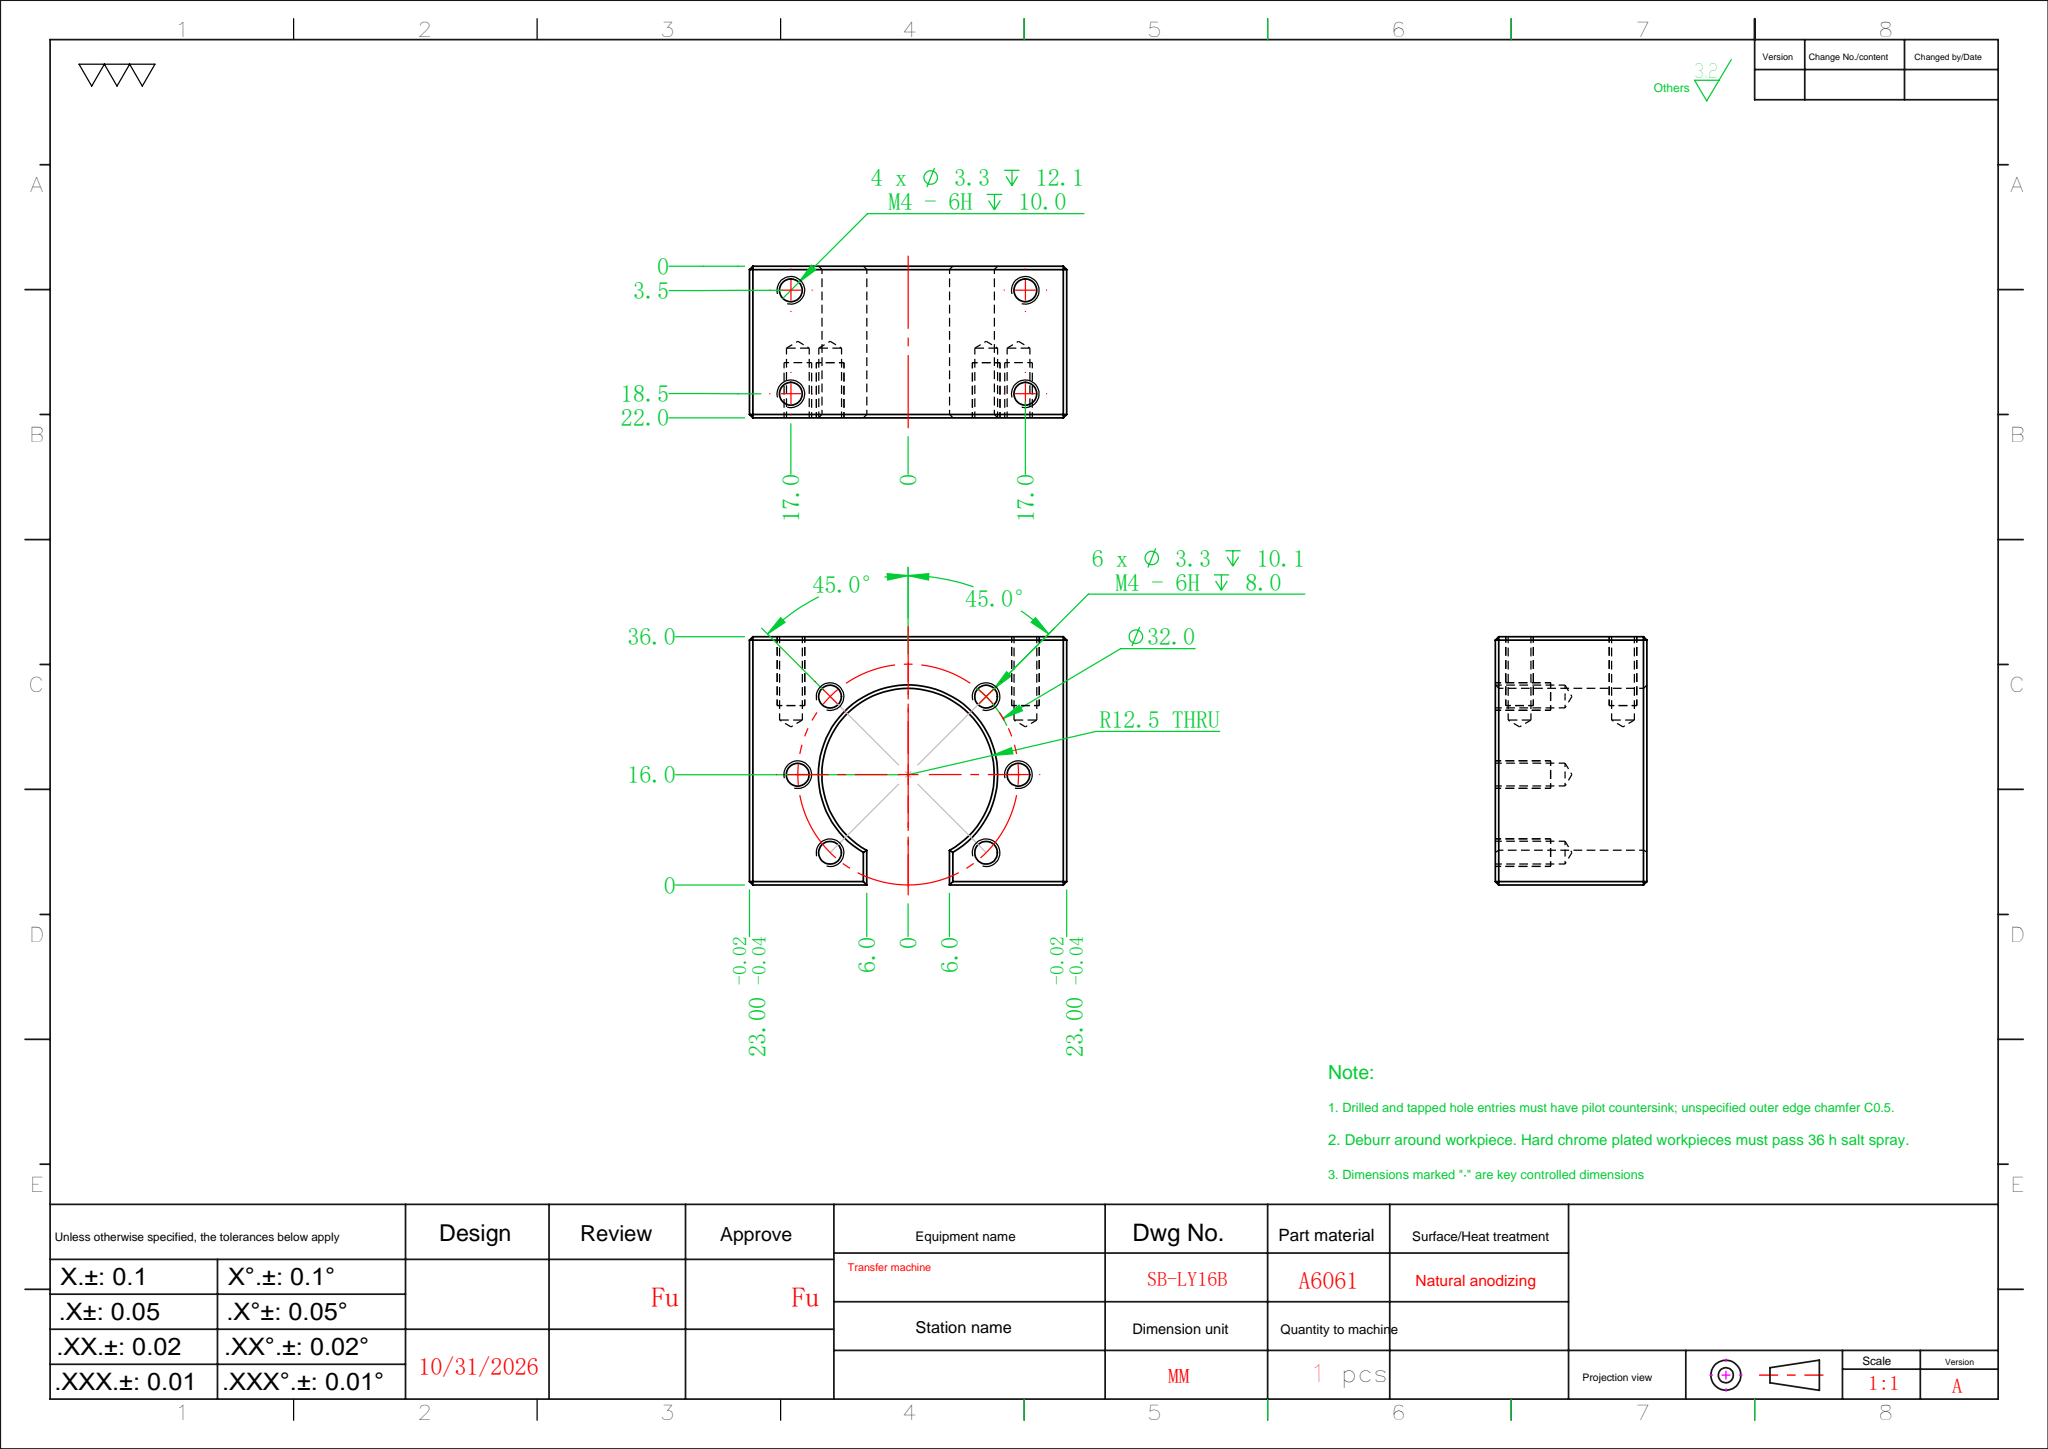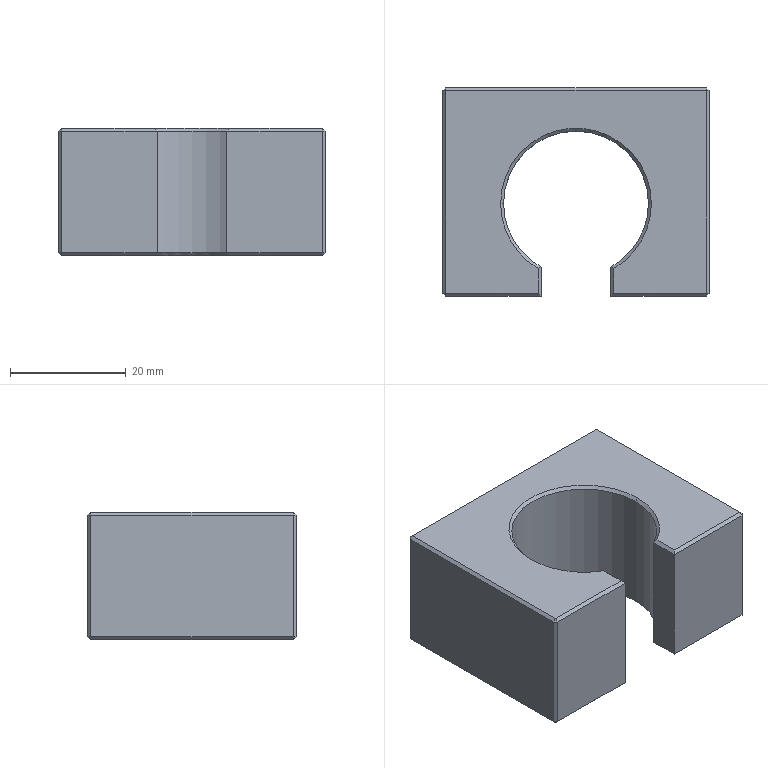Part | SolidWorks | features HoleWzd 2, Chamfer 1, Cut 1, Extrusion 1 | 1 solid | 84 faces | box 46 x 36 x 22 mm | volume 23549 mm3 | plane 35 | cone 26 | cylinder 23 | commonest cylinder face diameters 3.3 x20 25 x3